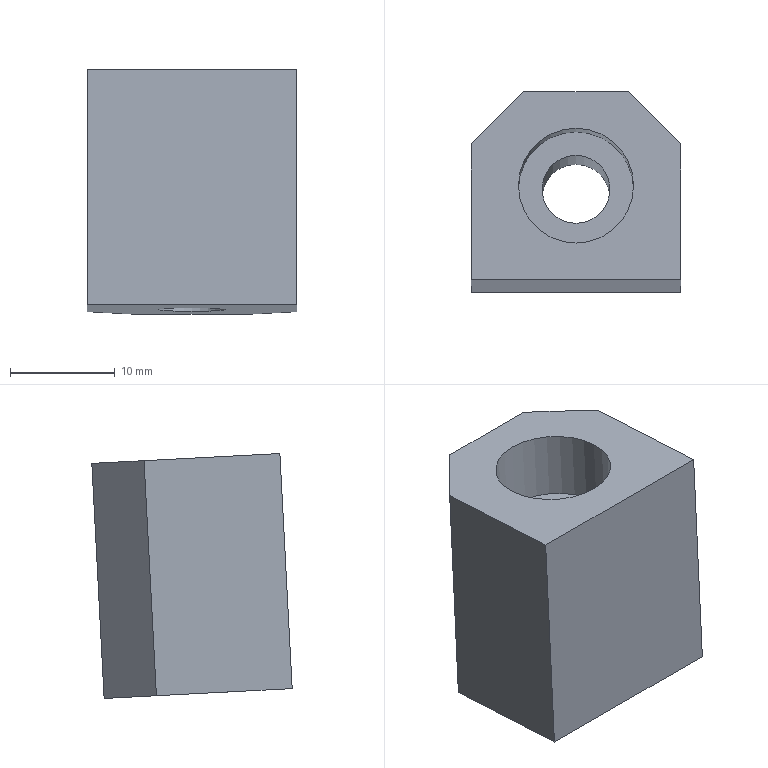Part | STEP file | P011002S001-007 | 1 solid | 11 faces | box 20 x 19.153 x 23.411 mm | volume 6389 mm3 | plane 9 | cylinder 2 | commonest cylinder face diameters 6.5 x1 11 x1
STEP:
#1=CARTESIAN_POINT('',(0.,0.,0.));
#2=DIRECTION('',(0.,0.,1.));
#3=DIRECTION('',(1.,0.,0.));
#4=AXIS2_PLACEMENT_3D('',#1,#2,#3);
#5=CARTESIAN_POINT('',(9.5,264.525,-24.398));
#6=VERTEX_POINT('',#5);
#7=CARTESIAN_POINT('',(9.5,277.507,-25.078));
#8=VERTEX_POINT('',#7);
#9=CARTESIAN_POINT('',(9.5,264.525,-24.398));
#10=DIRECTION('',(0.,0.9986,-0.05234));
#11=VECTOR('',#10,1.);
#12=LINE('',#9,#11);
#13=CARTESIAN_POINT('',(-5.5,264.525,-24.398));
#14=DIRECTION('',(0.,-0.05234,-0.9986));
#15=DIRECTION('',(0.,0.9986,-0.05234));
#16=AXIS2_PLACEMENT_3D('',#13,#14,#15);
#17=PLANE('',#16);
#18=CARTESIAN_POINT('',(0.,15.));
#19=DIRECTION('',(1.,0.));
#20=VECTOR('',#19,1.);
#21=LINE('',#18,#20);
#22=(GEOMETRIC_REPRESENTATION_CONTEXT(2)PARAMETRIC_REPRESENTATION_CONTEXT()REPRESENTATION_CONTEXT('',''));
#23=DEFINITIONAL_REPRESENTATION('',(#21),#22);
#24=PCURVE('',#17,#23);
#25=CARTESIAN_POINT('',(9.5,264.787,-19.405));
#26=DIRECTION('',(1.,0.,0.));
#27=DIRECTION('',(0.,-0.9986,0.05234));
#28=AXIS2_PLACEMENT_3D('',#25,#26,#27);
#29=PLANE('',#28);
#30=CARTESIAN_POINT('',(0.,5.));
#31=DIRECTION('',(-1.,0.));
#32=VECTOR('',#31,1.);
#33=LINE('',#30,#32);
#34=(GEOMETRIC_REPRESENTATION_CONTEXT(2)PARAMETRIC_REPRESENTATION_CONTEXT()REPRESENTATION_CONTEXT('',''));
#35=DEFINITIONAL_REPRESENTATION('',(#33),#34);
#36=PCURVE('',#29,#35);
#37=SURFACE_CURVE('',#12,(#24,#36),.PCURVE_S1.);
#38=EDGE_CURVE('',#6,#8,#37,.T.);
#39=ORIENTED_EDGE('',*,*,#38,.F.);
#40=CARTESIAN_POINT('',(-10.5,264.525,-24.398));
#41=VERTEX_POINT('',#40);
#42=CARTESIAN_POINT('',(-5.5,264.525,-24.398));
#43=DIRECTION('',(1.,0.,0.));
#44=VECTOR('',#43,1.);
#45=LINE('',#42,#44);
#46=CARTESIAN_POINT('',(0.,0.));
#47=DIRECTION('',(0.,1.));
#48=VECTOR('',#47,1.);
#49=LINE('',#46,#48);
#50=(GEOMETRIC_REPRESENTATION_CONTEXT(2)PARAMETRIC_REPRESENTATION_CONTEXT()REPRESENTATION_CONTEXT('',''));
#51=DEFINITIONAL_REPRESENTATION('',(#49),#50);
#52=PCURVE('',#17,#51);
#53=CARTESIAN_POINT('',(-5.5,264.787,-19.405));
#54=DIRECTION('',(0.,-0.9986,0.05234));
#55=DIRECTION('',(0.,-0.05234,-0.9986));
#56=AXIS2_PLACEMENT_3D('',#53,#54,#55);
#57=PLANE('',#56);
#58=CARTESIAN_POINT('',(5.,0.));
#59=DIRECTION('',(0.,1.));
#60=VECTOR('',#59,1.);
#61=LINE('',#58,#60);
#62=(GEOMETRIC_REPRESENTATION_CONTEXT(2)PARAMETRIC_REPRESENTATION_CONTEXT()REPRESENTATION_CONTEXT('',''));
#63=DEFINITIONAL_REPRESENTATION('',(#61),#62);
#64=PCURVE('',#57,#63);
#65=SURFACE_CURVE('',#45,(#52,#64),.PCURVE_S1.);
#66=EDGE_CURVE('',#41,#6,#65,.T.);
#67=ORIENTED_EDGE('',*,*,#66,.F.);
#68=CARTESIAN_POINT('',(-10.5,277.507,-25.078));
#69=VERTEX_POINT('',#68);
#70=CARTESIAN_POINT('',(-10.5,264.525,-24.398));
#71=DIRECTION('',(0.,0.9986,-0.05234));
#72=VECTOR('',#71,1.);
#73=LINE('',#70,#72);
#74=CARTESIAN_POINT('',(0.,-5.));
#75=DIRECTION('',(1.,0.));
#76=VECTOR('',#75,1.);
#77=LINE('',#74,#76);
#78=(GEOMETRIC_REPRESENTATION_CONTEXT(2)PARAMETRIC_REPRESENTATION_CONTEXT()REPRESENTATION_CONTEXT('',''));
#79=DEFINITIONAL_REPRESENTATION('',(#77),#78);
#80=PCURVE('',#17,#79);
#81=CARTESIAN_POINT('',(-10.5,264.787,-19.405));
#82=DIRECTION('',(-1.,0.,0.));
#83=DIRECTION('',(0.,0.9986,-0.05234));
#84=AXIS2_PLACEMENT_3D('',#81,#82,#83);
#85=PLANE('',#84);
#86=CARTESIAN_POINT('',(0.,5.));
#87=DIRECTION('',(1.,0.));
#88=VECTOR('',#87,1.);
#89=LINE('',#86,#88);
#90=(GEOMETRIC_REPRESENTATION_CONTEXT(2)PARAMETRIC_REPRESENTATION_CONTEXT()REPRESENTATION_CONTEXT('',''));
#91=DEFINITIONAL_REPRESENTATION('',(#89),#90);
#92=PCURVE('',#85,#91);
#93=SURFACE_CURVE('',#73,(#80,#92),.PCURVE_S1.);
#94=EDGE_CURVE('',#41,#69,#93,.T.);
#95=ORIENTED_EDGE('',*,*,#94,.T.);
#96=CARTESIAN_POINT('',(-5.5,282.5,-25.34));
#97=VERTEX_POINT('',#96);
#98=CARTESIAN_POINT('',(-14.5,273.513,-24.869));
#99=DIRECTION('',(-0.7071,-0.7061,0.03701));
#100=VECTOR('',#99,1.);
#101=LINE('',#98,#100);
#102=CARTESIAN_POINT('',(9.,-9.));
#103=DIRECTION('',(-0.7071,-0.7071));
#104=VECTOR('',#103,1.);
#105=LINE('',#102,#104);
#106=(GEOMETRIC_REPRESENTATION_CONTEXT(2)PARAMETRIC_REPRESENTATION_CONTEXT()REPRESENTATION_CONTEXT('',''));
#107=DEFINITIONAL_REPRESENTATION('',(#105),#106);
#108=PCURVE('',#17,#107);
#109=CARTESIAN_POINT('',(-10.5,277.769,-20.085));
#110=DIRECTION('',(0.7071,-0.7061,0.03701));
#111=DIRECTION('',(-0.7066,-0.7076,0.));
#112=AXIS2_PLACEMENT_3D('',#109,#110,#111);
#113=PLANE('',#112);
#114=CARTESIAN_POINT('',(5.838,4.787));
#115=DIRECTION('',(0.9993,-0.03703));
#116=VECTOR('',#115,1.);
#117=LINE('',#114,#116);
#118=(GEOMETRIC_REPRESENTATION_CONTEXT(2)PARAMETRIC_REPRESENTATION_CONTEXT()REPRESENTATION_CONTEXT('',''));
#119=DEFINITIONAL_REPRESENTATION('',(#117),#118);
#120=PCURVE('',#113,#119);
#121=SURFACE_CURVE('',#101,(#108,#120),.PCURVE_S1.);
#122=EDGE_CURVE('',#97,#69,#121,.T.);
#123=ORIENTED_EDGE('',*,*,#122,.F.);
#124=CARTESIAN_POINT('',(4.5,282.5,-25.34));
#125=VERTEX_POINT('',#124);
#126=CARTESIAN_POINT('',(-5.5,282.5,-25.34));
#127=DIRECTION('',(-1.,0.,0.));
#128=VECTOR('',#127,1.);
#129=LINE('',#126,#128);
#130=CARTESIAN_POINT('',(18.,0.));
#131=DIRECTION('',(0.,-1.));
#132=VECTOR('',#131,1.);
#133=LINE('',#130,#132);
#134=(GEOMETRIC_REPRESENTATION_CONTEXT(2)PARAMETRIC_REPRESENTATION_CONTEXT()REPRESENTATION_CONTEXT('',''));
#135=DEFINITIONAL_REPRESENTATION('',(#133),#134);
#136=PCURVE('',#17,#135);
#137=CARTESIAN_POINT('',(-5.5,282.762,-20.347));
#138=DIRECTION('',(0.,0.9986,-0.05234));
#139=DIRECTION('',(0.,0.05234,0.9986));
#140=AXIS2_PLACEMENT_3D('',#137,#138,#139);
#141=PLANE('',#140);
#142=CARTESIAN_POINT('',(-5.,0.));
#143=DIRECTION('',(0.,-1.));
#144=VECTOR('',#143,1.);
#145=LINE('',#142,#144);
#146=(GEOMETRIC_REPRESENTATION_CONTEXT(2)PARAMETRIC_REPRESENTATION_CONTEXT()REPRESENTATION_CONTEXT('',''));
#147=DEFINITIONAL_REPRESENTATION('',(#145),#146);
#148=PCURVE('',#141,#147);
#149=SURFACE_CURVE('',#129,(#136,#148),.PCURVE_S1.);
#150=EDGE_CURVE('',#125,#97,#149,.T.);
#151=ORIENTED_EDGE('',*,*,#150,.F.);
#152=CARTESIAN_POINT('',(8.5,278.506,-25.131));
#153=DIRECTION('',(-0.7071,0.7061,-0.03701));
#154=VECTOR('',#153,1.);
#155=LINE('',#152,#154);
#156=CARTESIAN_POINT('',(14.,14.));
#157=DIRECTION('',(0.7071,-0.7071));
#158=VECTOR('',#157,1.);
#159=LINE('',#156,#158);
#160=(GEOMETRIC_REPRESENTATION_CONTEXT(2)PARAMETRIC_REPRESENTATION_CONTEXT()REPRESENTATION_CONTEXT('',''));
#161=DEFINITIONAL_REPRESENTATION('',(#159),#160);
#162=PCURVE('',#17,#161);
#163=CARTESIAN_POINT('',(9.5,277.769,-20.085));
#164=DIRECTION('',(-0.7071,-0.7061,0.03701));
#165=DIRECTION('',(-0.7066,0.7076,0.));
#166=AXIS2_PLACEMENT_3D('',#163,#164,#165);
#167=PLANE('',#166);
#168=CARTESIAN_POINT('',(1.228,5.049));
#169=DIRECTION('',(0.9993,0.03703));
#170=VECTOR('',#169,1.);
#171=LINE('',#168,#170);
#172=(GEOMETRIC_REPRESENTATION_CONTEXT(2)PARAMETRIC_REPRESENTATION_CONTEXT()REPRESENTATION_CONTEXT('',''));
#173=DEFINITIONAL_REPRESENTATION('',(#171),#172);
#174=PCURVE('',#167,#173);
#175=SURFACE_CURVE('',#155,(#162,#174),.PCURVE_S1.);
#176=EDGE_CURVE('',#8,#125,#175,.T.);
#177=ORIENTED_EDGE('',*,*,#176,.F.);
#178=EDGE_LOOP('',(#39,#67,#95,#123,#151,#177));
#179=FACE_BOUND('',#178,.T.);
#180=CARTESIAN_POINT('',(-0.5,276.758,-25.039));
#181=VERTEX_POINT('',#180);
#182=CARTESIAN_POINT('',(-0.5,273.513,-24.869));
#183=DIRECTION('',(0.,-0.05234,-0.9986));
#184=DIRECTION('',(0.,0.9986,-0.05234));
#185=AXIS2_PLACEMENT_3D('',#182,#183,#184);
#186=CIRCLE('',#185,3.25);
#187=CARTESIAN_POINT('',(9.,5.));
#188=DIRECTION('',(1.,0.));
#189=AXIS2_PLACEMENT_2D('',#187,#188);
#190=CIRCLE('',#189,3.25);
#191=(GEOMETRIC_REPRESENTATION_CONTEXT(2)PARAMETRIC_REPRESENTATION_CONTEXT()REPRESENTATION_CONTEXT('',''));
#192=DEFINITIONAL_REPRESENTATION('',(#190),#191);
#193=PCURVE('',#17,#192);
#194=CARTESIAN_POINT('',(-0.5,274.69,-2.4));
#195=DIRECTION('',(0.,-0.05234,-0.9986));
#196=DIRECTION('',(0.,0.9986,-0.05234));
#197=AXIS2_PLACEMENT_3D('',#194,#195,#196);
#198=CYLINDRICAL_SURFACE('',#197,3.25);
#199=CARTESIAN_POINT('',(0.,22.5));
#200=DIRECTION('',(1.,0.));
#201=VECTOR('',#200,1.);
#202=LINE('',#199,#201);
#203=(GEOMETRIC_REPRESENTATION_CONTEXT(2)PARAMETRIC_REPRESENTATION_CONTEXT()REPRESENTATION_CONTEXT('',''));
#204=DEFINITIONAL_REPRESENTATION('',(#202),#203);
#205=PCURVE('',#198,#204);
#206=SURFACE_CURVE('',#186,(#193,#205),.PCURVE_S1.);
#207=EDGE_CURVE('',#181,#181,#206,.T.);
#208=ORIENTED_EDGE('',*,*,#207,.F.);
#209=EDGE_LOOP('',(#208));
#210=FACE_BOUND('',#209,.T.);
#211=ADVANCED_FACE('',(#179,#210),#17,.T.);
#212=ORIENTED_EDGE('',*,*,#150,.T.);
#213=CARTESIAN_POINT('',(-5.5,283.678,-2.871));
#214=VERTEX_POINT('',#213);
#215=CARTESIAN_POINT('',(-5.5,282.762,-20.347));
#216=DIRECTION('',(0.,-0.05234,-0.9986));
#217=VECTOR('',#216,1.);
#218=LINE('',#215,#217);
#219=CARTESIAN_POINT('',(0.,0.));
#220=DIRECTION('',(-1.,0.));
#221=VECTOR('',#220,1.);
#222=LINE('',#219,#221);
#223=(GEOMETRIC_REPRESENTATION_CONTEXT(2)PARAMETRIC_REPRESENTATION_CONTEXT()REPRESENTATION_CONTEXT('',''));
#224=DEFINITIONAL_REPRESENTATION('',(#222),#223);
#225=PCURVE('',#141,#224);
#226=CARTESIAN_POINT('',(-7.066,0.2619));
#227=DIRECTION('',(0.03703,0.9993));
#228=VECTOR('',#227,1.);
#229=LINE('',#226,#228);
#230=(GEOMETRIC_REPRESENTATION_CONTEXT(2)PARAMETRIC_REPRESENTATION_CONTEXT()REPRESENTATION_CONTEXT('',''));
#231=DEFINITIONAL_REPRESENTATION('',(#229),#230);
#232=PCURVE('',#113,#231);
#233=SURFACE_CURVE('',#218,(#225,#232),.PCURVE_S1.);
#234=EDGE_CURVE('',#214,#97,#233,.T.);
#235=ORIENTED_EDGE('',*,*,#234,.F.);
#236=CARTESIAN_POINT('',(4.5,283.678,-2.871));
#237=VERTEX_POINT('',#236);
#238=CARTESIAN_POINT('',(-5.5,283.678,-2.871));
#239=DIRECTION('',(1.,0.,0.));
#240=VECTOR('',#239,1.);
#241=LINE('',#238,#240);
#242=CARTESIAN_POINT('',(17.5,0.));
#243=DIRECTION('',(0.,1.));
#244=VECTOR('',#243,1.);
#245=LINE('',#242,#244);
#246=(GEOMETRIC_REPRESENTATION_CONTEXT(2)PARAMETRIC_REPRESENTATION_CONTEXT()REPRESENTATION_CONTEXT('',''));
#247=DEFINITIONAL_REPRESENTATION('',(#245),#246);
#248=PCURVE('',#141,#247);
#249=CARTESIAN_POINT('',(-5.5,265.703,-1.929));
#250=DIRECTION('',(0.,0.05234,0.9986));
#251=DIRECTION('',(0.,-0.9986,0.05234));
#252=AXIS2_PLACEMENT_3D('',#249,#250,#251);
#253=PLANE('',#252);
#254=CARTESIAN_POINT('',(-18.,0.));
#255=DIRECTION('',(0.,1.));
#256=VECTOR('',#255,1.);
#257=LINE('',#254,#256);
#258=(GEOMETRIC_REPRESENTATION_CONTEXT(2)PARAMETRIC_REPRESENTATION_CONTEXT()REPRESENTATION_CONTEXT('',''));
#259=DEFINITIONAL_REPRESENTATION('',(#257),#258);
#260=PCURVE('',#253,#259);
#261=SURFACE_CURVE('',#241,(#248,#260),.PCURVE_S1.);
#262=EDGE_CURVE('',#214,#237,#261,.T.);
#263=ORIENTED_EDGE('',*,*,#262,.T.);
#264=CARTESIAN_POINT('',(4.5,282.762,-20.347));
#265=DIRECTION('',(0.,0.05234,0.9986));
#266=VECTOR('',#265,1.);
#267=LINE('',#264,#266);
#268=CARTESIAN_POINT('',(0.,10.));
#269=DIRECTION('',(1.,0.));
#270=VECTOR('',#269,1.);
#271=LINE('',#268,#270);
#272=(GEOMETRIC_REPRESENTATION_CONTEXT(2)PARAMETRIC_REPRESENTATION_CONTEXT()REPRESENTATION_CONTEXT('',''));
#273=DEFINITIONAL_REPRESENTATION('',(#271),#272);
#274=PCURVE('',#141,#273);
#275=CARTESIAN_POINT('',(7.066,0.2619));
#276=DIRECTION('',(0.03703,-0.9993));
#277=VECTOR('',#276,1.);
#278=LINE('',#275,#277);
#279=(GEOMETRIC_REPRESENTATION_CONTEXT(2)PARAMETRIC_REPRESENTATION_CONTEXT()REPRESENTATION_CONTEXT('',''));
#280=DEFINITIONAL_REPRESENTATION('',(#278),#279);
#281=PCURVE('',#167,#280);
#282=SURFACE_CURVE('',#267,(#274,#281),.PCURVE_S1.);
#283=EDGE_CURVE('',#125,#237,#282,.T.);
#284=ORIENTED_EDGE('',*,*,#283,.F.);
#285=EDGE_LOOP('',(#212,#235,#263,#284));
#286=FACE_BOUND('',#285,.T.);
#287=ADVANCED_FACE('',(#286),#141,.T.);
#288=CARTESIAN_POINT('',(9.5,265.703,-1.929));
#289=VERTEX_POINT('',#288);
#290=CARTESIAN_POINT('',(9.5,278.685,-2.609));
#291=VERTEX_POINT('',#290);
#292=CARTESIAN_POINT('',(9.5,265.703,-1.929));
#293=DIRECTION('',(0.,0.9986,-0.05234));
#294=VECTOR('',#293,1.);
#295=LINE('',#292,#294);
#296=CARTESIAN_POINT('',(0.,-17.5));
#297=DIRECTION('',(-1.,0.));
#298=VECTOR('',#297,1.);
#299=LINE('',#296,#298);
#300=(GEOMETRIC_REPRESENTATION_CONTEXT(2)PARAMETRIC_REPRESENTATION_CONTEXT()REPRESENTATION_CONTEXT('',''));
#301=DEFINITIONAL_REPRESENTATION('',(#299),#300);
#302=PCURVE('',#29,#301);
#303=CARTESIAN_POINT('',(0.,15.));
#304=DIRECTION('',(-1.,0.));
#305=VECTOR('',#304,1.);
#306=LINE('',#303,#305);
#307=(GEOMETRIC_REPRESENTATION_CONTEXT(2)PARAMETRIC_REPRESENTATION_CONTEXT()REPRESENTATION_CONTEXT('',''));
#308=DEFINITIONAL_REPRESENTATION('',(#306),#307);
#309=PCURVE('',#253,#308);
#310=SURFACE_CURVE('',#295,(#302,#309),.PCURVE_S1.);
#311=EDGE_CURVE('',#289,#291,#310,.T.);
#312=ORIENTED_EDGE('',*,*,#311,.F.);
#313=CARTESIAN_POINT('',(9.5,264.787,-19.405));
#314=DIRECTION('',(0.,0.05234,0.9986));
#315=VECTOR('',#314,1.);
#316=LINE('',#313,#315);
#317=CARTESIAN_POINT('',(0.,0.));
#318=DIRECTION('',(0.,-1.));
#319=VECTOR('',#318,1.);
#320=LINE('',#317,#319);
#321=(GEOMETRIC_REPRESENTATION_CONTEXT(2)PARAMETRIC_REPRESENTATION_CONTEXT()REPRESENTATION_CONTEXT('',''));
#322=DEFINITIONAL_REPRESENTATION('',(#320),#321);
#323=PCURVE('',#29,#322);
#324=CARTESIAN_POINT('',(0.,15.));
#325=DIRECTION('',(-1.,0.));
#326=VECTOR('',#325,1.);
#327=LINE('',#324,#326);
#328=(GEOMETRIC_REPRESENTATION_CONTEXT(2)PARAMETRIC_REPRESENTATION_CONTEXT()REPRESENTATION_CONTEXT('',''));
#329=DEFINITIONAL_REPRESENTATION('',(#327),#328);
#330=PCURVE('',#57,#329);
#331=SURFACE_CURVE('',#316,(#323,#330),.PCURVE_S1.);
#332=EDGE_CURVE('',#6,#289,#331,.T.);
#333=ORIENTED_EDGE('',*,*,#332,.F.);
#334=ORIENTED_EDGE('',*,*,#38,.T.);
#335=CARTESIAN_POINT('',(9.5,277.769,-20.085));
#336=DIRECTION('',(0.,-0.05234,-0.9986));
#337=VECTOR('',#336,1.);
#338=LINE('',#335,#337);
#339=CARTESIAN_POINT('',(-13.,0.));
#340=DIRECTION('',(0.,1.));
#341=VECTOR('',#340,1.);
#342=LINE('',#339,#341);
#343=(GEOMETRIC_REPRESENTATION_CONTEXT(2)PARAMETRIC_REPRESENTATION_CONTEXT()REPRESENTATION_CONTEXT('',''));
#344=DEFINITIONAL_REPRESENTATION('',(#342),#343);
#345=PCURVE('',#29,#344);
#346=CARTESIAN_POINT('',(0.,0.));
#347=DIRECTION('',(-0.03703,0.9993));
#348=VECTOR('',#347,1.);
#349=LINE('',#346,#348);
#350=(GEOMETRIC_REPRESENTATION_CONTEXT(2)PARAMETRIC_REPRESENTATION_CONTEXT()REPRESENTATION_CONTEXT('',''));
#351=DEFINITIONAL_REPRESENTATION('',(#349),#350);
#352=PCURVE('',#167,#351);
#353=SURFACE_CURVE('',#338,(#345,#352),.PCURVE_S1.);
#354=EDGE_CURVE('',#291,#8,#353,.T.);
#355=ORIENTED_EDGE('',*,*,#354,.F.);
#356=EDGE_LOOP('',(#312,#333,#334,#355));
#357=FACE_BOUND('',#356,.T.);
#358=ADVANCED_FACE('',(#357),#29,.T.);
#359=ORIENTED_EDGE('',*,*,#94,.F.);
#360=CARTESIAN_POINT('',(-10.5,265.703,-1.929));
#361=VERTEX_POINT('',#360);
#362=CARTESIAN_POINT('',(-10.5,264.787,-19.405));
#363=DIRECTION('',(0.,-0.05234,-0.9986));
#364=VECTOR('',#363,1.);
#365=LINE('',#362,#364);
#366=CARTESIAN_POINT('',(0.,0.));
#367=DIRECTION('',(0.,1.));
#368=VECTOR('',#367,1.);
#369=LINE('',#366,#368);
#370=(GEOMETRIC_REPRESENTATION_CONTEXT(2)PARAMETRIC_REPRESENTATION_CONTEXT()REPRESENTATION_CONTEXT('',''));
#371=DEFINITIONAL_REPRESENTATION('',(#369),#370);
#372=PCURVE('',#85,#371);
#373=CARTESIAN_POINT('',(0.,-5.));
#374=DIRECTION('',(1.,0.));
#375=VECTOR('',#374,1.);
#376=LINE('',#373,#375);
#377=(GEOMETRIC_REPRESENTATION_CONTEXT(2)PARAMETRIC_REPRESENTATION_CONTEXT()REPRESENTATION_CONTEXT('',''));
#378=DEFINITIONAL_REPRESENTATION('',(#376),#377);
#379=PCURVE('',#57,#378);
#380=SURFACE_CURVE('',#365,(#372,#379),.PCURVE_S1.);
#381=EDGE_CURVE('',#361,#41,#380,.T.);
#382=ORIENTED_EDGE('',*,*,#381,.F.);
#383=CARTESIAN_POINT('',(-10.5,278.685,-2.609));
#384=VERTEX_POINT('',#383);
#385=CARTESIAN_POINT('',(-10.5,265.703,-1.929));
#386=DIRECTION('',(0.,0.9986,-0.05234));
#387=VECTOR('',#386,1.);
#388=LINE('',#385,#387);
#389=CARTESIAN_POINT('',(0.,-17.5));
#390=DIRECTION('',(1.,0.));
#391=VECTOR('',#390,1.);
#392=LINE('',#389,#391);
#393=(GEOMETRIC_REPRESENTATION_CONTEXT(2)PARAMETRIC_REPRESENTATION_CONTEXT()REPRESENTATION_CONTEXT('',''));
#394=DEFINITIONAL_REPRESENTATION('',(#392),#393);
#395=PCURVE('',#85,#394);
#396=CARTESIAN_POINT('',(0.,-5.));
#397=DIRECTION('',(-1.,0.));
#398=VECTOR('',#397,1.);
#399=LINE('',#396,#398);
#400=(GEOMETRIC_REPRESENTATION_CONTEXT(2)PARAMETRIC_REPRESENTATION_CONTEXT()REPRESENTATION_CONTEXT('',''));
#401=DEFINITIONAL_REPRESENTATION('',(#399),#400);
#402=PCURVE('',#253,#401);
#403=SURFACE_CURVE('',#388,(#395,#402),.PCURVE_S1.);
#404=EDGE_CURVE('',#361,#384,#403,.T.);
#405=ORIENTED_EDGE('',*,*,#404,.T.);
#406=CARTESIAN_POINT('',(-10.5,277.769,-20.085));
#407=DIRECTION('',(0.,0.05234,0.9986));
#408=VECTOR('',#407,1.);
#409=LINE('',#406,#408);
#410=CARTESIAN_POINT('',(13.,0.));
#411=DIRECTION('',(0.,-1.));
#412=VECTOR('',#411,1.);
#413=LINE('',#410,#412);
#414=(GEOMETRIC_REPRESENTATION_CONTEXT(2)PARAMETRIC_REPRESENTATION_CONTEXT()REPRESENTATION_CONTEXT('',''));
#415=DEFINITIONAL_REPRESENTATION('',(#413),#414);
#416=PCURVE('',#85,#415);
#417=CARTESIAN_POINT('',(0.,0.));
#418=DIRECTION('',(-0.03703,-0.9993));
#419=VECTOR('',#418,1.);
#420=LINE('',#417,#419);
#421=(GEOMETRIC_REPRESENTATION_CONTEXT(2)PARAMETRIC_REPRESENTATION_CONTEXT()REPRESENTATION_CONTEXT('',''));
#422=DEFINITIONAL_REPRESENTATION('',(#420),#421);
#423=PCURVE('',#113,#422);
#424=SURFACE_CURVE('',#409,(#416,#423),.PCURVE_S1.);
#425=EDGE_CURVE('',#69,#384,#424,.T.);
#426=ORIENTED_EDGE('',*,*,#425,.F.);
#427=EDGE_LOOP('',(#359,#382,#405,#426));
#428=FACE_BOUND('',#427,.T.);
#429=ADVANCED_FACE('',(#428),#85,.T.);
#430=CARTESIAN_POINT('',(-5.5,265.703,-1.929));
#431=DIRECTION('',(-1.,0.,0.));
#432=VECTOR('',#431,1.);
#433=LINE('',#430,#432);
#434=CARTESIAN_POINT('',(-17.5,0.));
#435=DIRECTION('',(0.,-1.));
#436=VECTOR('',#435,1.);
#437=LINE('',#434,#436);
#438=(GEOMETRIC_REPRESENTATION_CONTEXT(2)PARAMETRIC_REPRESENTATION_CONTEXT()REPRESENTATION_CONTEXT('',''));
#439=DEFINITIONAL_REPRESENTATION('',(#437),#438);
#440=PCURVE('',#57,#439);
#441=CARTESIAN_POINT('',(0.,0.));
#442=DIRECTION('',(0.,-1.));
#443=VECTOR('',#442,1.);
#444=LINE('',#441,#443);
#445=(GEOMETRIC_REPRESENTATION_CONTEXT(2)PARAMETRIC_REPRESENTATION_CONTEXT()REPRESENTATION_CONTEXT('',''));
#446=DEFINITIONAL_REPRESENTATION('',(#444),#445);
#447=PCURVE('',#253,#446);
#448=SURFACE_CURVE('',#433,(#440,#447),.PCURVE_S1.);
#449=EDGE_CURVE('',#289,#361,#448,.T.);
#450=ORIENTED_EDGE('',*,*,#449,.T.);
#451=ORIENTED_EDGE('',*,*,#381,.T.);
#452=ORIENTED_EDGE('',*,*,#66,.T.);
#453=ORIENTED_EDGE('',*,*,#332,.T.);
#454=EDGE_LOOP('',(#450,#451,#452,#453));
#455=FACE_BOUND('',#454,.T.);
#456=ADVANCED_FACE('',(#455),#57,.T.);
#457=CARTESIAN_POINT('',(-0.5,269.198,-2.112));
#458=VERTEX_POINT('',#457);
#459=CARTESIAN_POINT('',(-0.5,280.183,-2.688));
#460=VERTEX_POINT('',#459);
#461=CARTESIAN_POINT('',(-0.5,274.69,-2.4));
#462=DIRECTION('',(0.,-0.05234,-0.9986));
#463=DIRECTION('',(0.,-0.9986,0.05234));
#464=AXIS2_PLACEMENT_3D('',#461,#462,#463);
#465=CIRCLE('',#464,5.5);
#466=CARTESIAN_POINT('',(-3.5,5.));
#467=CARTESIAN_POINT('',(-3.5,-4.526));
#468=CARTESIAN_POINT('',(-11.75,0.2369));
#469=CARTESIAN_POINT('',(-20.,5.));
#470=CARTESIAN_POINT('',(-11.75,9.763));
#471=CARTESIAN_POINT('',(-3.5,14.526));
#472=CARTESIAN_POINT('',(-3.5,5.));
#473=(BOUNDED_CURVE()B_SPLINE_CURVE(2,(#466,#467,#468,#469,#470,#471,#472),.UNSPECIFIED.,.T.,.F.)B_SPLINE_CURVE_WITH_KNOTS((1,2,2,2,2,1),(-2.094,0.,2.094,4.189,6.283,8.378),.UNSPECIFIED.)CURVE()GEOMETRIC_REPRESENTATION_ITEM()RATIONAL_B_SPLINE_CURVE((1.,0.5,1.,0.5,1.,0.5,1.))REPRESENTATION_ITEM(''));
#474=(GEOMETRIC_REPRESENTATION_CONTEXT(2)PARAMETRIC_REPRESENTATION_CONTEXT()REPRESENTATION_CONTEXT('',''));
#475=DEFINITIONAL_REPRESENTATION('',(#473),#474);
#476=PCURVE('',#253,#475);
#477=CARTESIAN_POINT('',(-0.5,274.69,-2.4));
#478=DIRECTION('',(0.,-0.05234,-0.9986));
#479=DIRECTION('',(0.,0.9986,-0.05234));
#480=AXIS2_PLACEMENT_3D('',#477,#478,#479);
#481=CYLINDRICAL_SURFACE('',#480,5.5);
#482=CARTESIAN_POINT('',(3.142,0.));
#483=DIRECTION('',(1.,0.));
#484=VECTOR('',#483,1.);
#485=LINE('',#482,#484);
#486=(GEOMETRIC_REPRESENTATION_CONTEXT(2)PARAMETRIC_REPRESENTATION_CONTEXT()REPRESENTATION_CONTEXT('',''));
#487=DEFINITIONAL_REPRESENTATION('',(#485),#486);
#488=PCURVE('',#481,#487);
#489=SURFACE_CURVE('',#465,(#476,#488),.PCURVE_S1.);
#490=EDGE_CURVE('',#458,#460,#489,.T.);
#491=ORIENTED_EDGE('',*,*,#490,.T.);
#492=CARTESIAN_POINT('',(-0.5,274.69,-2.4));
#493=DIRECTION('',(0.,-0.05234,-0.9986));
#494=DIRECTION('',(0.,-0.9986,0.05234));
#495=AXIS2_PLACEMENT_3D('',#492,#493,#494);
#496=CIRCLE('',#495,5.5);
#497=CARTESIAN_POINT('',(-3.5,5.));
#498=CARTESIAN_POINT('',(-3.5,-4.526));
#499=CARTESIAN_POINT('',(-11.75,0.2369));
#500=CARTESIAN_POINT('',(-20.,5.));
#501=CARTESIAN_POINT('',(-11.75,9.763));
#502=CARTESIAN_POINT('',(-3.5,14.526));
#503=CARTESIAN_POINT('',(-3.5,5.));
#504=(BOUNDED_CURVE()B_SPLINE_CURVE(2,(#497,#498,#499,#500,#501,#502,#503),.UNSPECIFIED.,.T.,.F.)B_SPLINE_CURVE_WITH_KNOTS((1,2,2,2,2,1),(-2.094,0.,2.094,4.189,6.283,8.378),.UNSPECIFIED.)CURVE()GEOMETRIC_REPRESENTATION_ITEM()RATIONAL_B_SPLINE_CURVE((1.,0.5,1.,0.5,1.,0.5,1.))REPRESENTATION_ITEM(''));
#505=(GEOMETRIC_REPRESENTATION_CONTEXT(2)PARAMETRIC_REPRESENTATION_CONTEXT()REPRESENTATION_CONTEXT('',''));
#506=DEFINITIONAL_REPRESENTATION('',(#504),#505);
#507=PCURVE('',#253,#506);
#508=CARTESIAN_POINT('',(-3.142,0.));
#509=DIRECTION('',(1.,0.));
#510=VECTOR('',#509,1.);
#511=LINE('',#508,#510);
#512=(GEOMETRIC_REPRESENTATION_CONTEXT(2)PARAMETRIC_REPRESENTATION_CONTEXT()REPRESENTATION_CONTEXT('',''));
#513=DEFINITIONAL_REPRESENTATION('',(#511),#512);
#514=PCURVE('',#481,#513);
#515=SURFACE_CURVE('',#496,(#507,#514),.PCURVE_S1.);
#516=EDGE_CURVE('',#460,#458,#515,.T.);
#517=ORIENTED_EDGE('',*,*,#516,.T.);
#518=EDGE_LOOP('',(#491,#517));
#519=FACE_BOUND('',#518,.T.);
#520=ORIENTED_EDGE('',*,*,#262,.F.);
#521=CARTESIAN_POINT('',(-14.5,274.69,-2.4));
#522=DIRECTION('',(0.7071,0.7061,-0.03701));
#523=VECTOR('',#522,1.);
#524=LINE('',#521,#523);
#525=CARTESIAN_POINT('',(-9.,-9.));
#526=DIRECTION('',(-0.7071,0.7071));
#527=VECTOR('',#526,1.);
#528=LINE('',#525,#527);
#529=(GEOMETRIC_REPRESENTATION_CONTEXT(2)PARAMETRIC_REPRESENTATION_CONTEXT()REPRESENTATION_CONTEXT('',''));
#530=DEFINITIONAL_REPRESENTATION('',(#528),#529);
#531=PCURVE('',#253,#530);
#532=CARTESIAN_POINT('',(5.005,-17.697));
#533=DIRECTION('',(-0.9993,0.03703));
#534=VECTOR('',#533,1.);
#535=LINE('',#532,#534);
#536=(GEOMETRIC_REPRESENTATION_CONTEXT(2)PARAMETRIC_REPRESENTATION_CONTEXT()REPRESENTATION_CONTEXT('',''));
#537=DEFINITIONAL_REPRESENTATION('',(#535),#536);
#538=PCURVE('',#113,#537);
#539=SURFACE_CURVE('',#524,(#531,#538),.PCURVE_S1.);
#540=EDGE_CURVE('',#384,#214,#539,.T.);
#541=ORIENTED_EDGE('',*,*,#540,.F.);
#542=ORIENTED_EDGE('',*,*,#404,.F.);
#543=ORIENTED_EDGE('',*,*,#449,.F.);
#544=ORIENTED_EDGE('',*,*,#311,.T.);
#545=CARTESIAN_POINT('',(8.5,279.683,-2.662));
#546=DIRECTION('',(0.7071,-0.7061,0.03701));
#547=VECTOR('',#546,1.);
#548=LINE('',#545,#547);
#549=CARTESIAN_POINT('',(-14.,14.));
#550=DIRECTION('',(0.7071,0.7071));
#551=VECTOR('',#550,1.);
#552=LINE('',#549,#551);
#553=(GEOMETRIC_REPRESENTATION_CONTEXT(2)PARAMETRIC_REPRESENTATION_CONTEXT()REPRESENTATION_CONTEXT('',''));
#554=DEFINITIONAL_REPRESENTATION('',(#552),#553);
#555=PCURVE('',#253,#554);
#556=CARTESIAN_POINT('',(2.061,-17.436));
#557=DIRECTION('',(-0.9993,-0.03703));
#558=VECTOR('',#557,1.);
#559=LINE('',#556,#558);
#560=(GEOMETRIC_REPRESENTATION_CONTEXT(2)PARAMETRIC_REPRESENTATION_CONTEXT()REPRESENTATION_CONTEXT('',''));
#561=DEFINITIONAL_REPRESENTATION('',(#559),#560);
#562=PCURVE('',#167,#561);
#563=SURFACE_CURVE('',#548,(#555,#562),.PCURVE_S1.);
#564=EDGE_CURVE('',#237,#291,#563,.T.);
#565=ORIENTED_EDGE('',*,*,#564,.F.);
#566=EDGE_LOOP('',(#520,#541,#542,#543,#544,#565));
#567=FACE_BOUND('',#566,.T.);
#568=ADVANCED_FACE('',(#519,#567),#253,.T.);
#569=ORIENTED_EDGE('',*,*,#564,.T.);
#570=ORIENTED_EDGE('',*,*,#354,.T.);
#571=ORIENTED_EDGE('',*,*,#176,.T.);
#572=ORIENTED_EDGE('',*,*,#283,.T.);
#573=EDGE_LOOP('',(#569,#570,#571,#572));
#574=FACE_BOUND('',#573,.T.);
#575=ADVANCED_FACE('',(#574),#167,.F.);
#576=ORIENTED_EDGE('',*,*,#122,.T.);
#577=ORIENTED_EDGE('',*,*,#425,.T.);
#578=ORIENTED_EDGE('',*,*,#540,.T.);
#579=ORIENTED_EDGE('',*,*,#234,.T.);
#580=EDGE_LOOP('',(#576,#577,#578,#579));
#581=FACE_BOUND('',#580,.T.);
#582=ADVANCED_FACE('',(#581),#113,.F.);
#583=ORIENTED_EDGE('',*,*,#207,.F.);
#584=CARTESIAN_POINT('',(-0.5,277.596,-9.061));
#585=VERTEX_POINT('',#584);
#586=CARTESIAN_POINT('',(-0.5,277.596,-9.061));
#587=CARTESIAN_POINT('',(-0.5,276.758,-25.039));
#588=B_SPLINE_CURVE_WITH_KNOTS('',1,(#586,#587),.UNSPECIFIED.,.F.,.F.,(2,2),(6.5,22.5),.PIECEWISE_BEZIER_KNOTS.);
#589=CARTESIAN_POINT('',(0.,0.));
#590=DIRECTION('',(0.,1.));
#591=VECTOR('',#590,1.);
#592=LINE('',#589,#591);
#593=(GEOMETRIC_REPRESENTATION_CONTEXT(2)PARAMETRIC_REPRESENTATION_CONTEXT()REPRESENTATION_CONTEXT('',''));
#594=DEFINITIONAL_REPRESENTATION('',(#592),#593);
#595=PCURVE('',#198,#594);
#596=CARTESIAN_POINT('',(6.283,0.));
#597=DIRECTION('',(0.,1.));
#598=VECTOR('',#597,1.);
#599=LINE('',#596,#598);
#600=(GEOMETRIC_REPRESENTATION_CONTEXT(2)PARAMETRIC_REPRESENTATION_CONTEXT()REPRESENTATION_CONTEXT('',''));
#601=DEFINITIONAL_REPRESENTATION('',(#599),#600);
#602=PCURVE('',#198,#601);
#603=SEAM_CURVE('',#588,(#595,#602),.PCURVE_S1.);
#604=EDGE_CURVE('',#585,#181,#603,.T.);
#605=ORIENTED_EDGE('',*,*,#604,.F.);
#606=CARTESIAN_POINT('',(-0.5,274.35,-8.891));
#607=DIRECTION('',(0.,0.05234,0.9986));
#608=DIRECTION('',(0.,0.9986,-0.05234));
#609=AXIS2_PLACEMENT_3D('',#606,#607,#608);
#610=CIRCLE('',#609,3.25);
#611=CARTESIAN_POINT('',(6.283,6.5));
#612=DIRECTION('',(-1.,0.));
#613=VECTOR('',#612,1.);
#614=LINE('',#611,#613);
#615=(GEOMETRIC_REPRESENTATION_CONTEXT(2)PARAMETRIC_REPRESENTATION_CONTEXT()REPRESENTATION_CONTEXT('',''));
#616=DEFINITIONAL_REPRESENTATION('',(#614),#615);
#617=PCURVE('',#198,#616);
#618=CARTESIAN_POINT('',(-0.5,274.35,-8.891));
#619=DIRECTION('',(0.,-0.05234,-0.9986));
#620=DIRECTION('',(0.,0.9986,-0.05234));
#621=AXIS2_PLACEMENT_3D('',#618,#619,#620);
#622=PLANE('',#621);
#623=CARTESIAN_POINT('',(3.25,0.));
#624=CARTESIAN_POINT('',(3.25,-5.629));
#625=CARTESIAN_POINT('',(-1.625,-2.815));
#626=CARTESIAN_POINT('',(-6.5,0.));
#627=CARTESIAN_POINT('',(-1.625,2.815));
#628=CARTESIAN_POINT('',(3.25,5.629));
#629=CARTESIAN_POINT('',(3.25,0.));
#630=(BOUNDED_CURVE()B_SPLINE_CURVE(2,(#623,#624,#625,#626,#627,#628,#629),.UNSPECIFIED.,.T.,.F.)B_SPLINE_CURVE_WITH_KNOTS((1,2,2,2,2,1),(-2.094,0.,2.094,4.189,6.283,8.378),.UNSPECIFIED.)CURVE()GEOMETRIC_REPRESENTATION_ITEM()RATIONAL_B_SPLINE_CURVE((1.,0.5,1.,0.5,1.,0.5,1.))REPRESENTATION_ITEM(''));
#631=(GEOMETRIC_REPRESENTATION_CONTEXT(2)PARAMETRIC_REPRESENTATION_CONTEXT()REPRESENTATION_CONTEXT('',''));
#632=DEFINITIONAL_REPRESENTATION('',(#630),#631);
#633=PCURVE('',#622,#632);
#634=SURFACE_CURVE('',#610,(#617,#633),.PCURVE_S1.);
#635=EDGE_CURVE('',#585,#585,#634,.T.);
#636=ORIENTED_EDGE('',*,*,#635,.F.);
#637=ORIENTED_EDGE('',*,*,#604,.T.);
#638=EDGE_LOOP('',(#583,#605,#636,#637));
#639=FACE_BOUND('',#638,.F.);
#640=ADVANCED_FACE('',(#639),#198,.F.);
#641=CARTESIAN_POINT('',(-0.5,279.843,-9.179));
#642=VERTEX_POINT('',#641);
#643=CARTESIAN_POINT('',(-0.5,274.35,-8.891));
#644=DIRECTION('',(0.,0.05234,0.9986));
#645=DIRECTION('',(0.,0.9986,-0.05234));
#646=AXIS2_PLACEMENT_3D('',#643,#644,#645);
#647=CIRCLE('',#646,5.5);
#648=CARTESIAN_POINT('',(5.5,0.));
#649=CARTESIAN_POINT('',(5.5,-9.526));
#650=CARTESIAN_POINT('',(-2.75,-4.763));
#651=CARTESIAN_POINT('',(-11.,0.));
#652=CARTESIAN_POINT('',(-2.75,4.763));
#653=CARTESIAN_POINT('',(5.5,9.526));
#654=CARTESIAN_POINT('',(5.5,0.));
#655=(BOUNDED_CURVE()B_SPLINE_CURVE(2,(#648,#649,#650,#651,#652,#653,#654),.UNSPECIFIED.,.T.,.F.)B_SPLINE_CURVE_WITH_KNOTS((1,2,2,2,2,1),(-2.094,0.,2.094,4.189,6.283,8.378),.UNSPECIFIED.)CURVE()GEOMETRIC_REPRESENTATION_ITEM()RATIONAL_B_SPLINE_CURVE((1.,0.5,1.,0.5,1.,0.5,1.))REPRESENTATION_ITEM(''));
#656=(GEOMETRIC_REPRESENTATION_CONTEXT(2)PARAMETRIC_REPRESENTATION_CONTEXT()REPRESENTATION_CONTEXT('',''));
#657=DEFINITIONAL_REPRESENTATION('',(#655),#656);
#658=PCURVE('',#622,#657);
#659=CARTESIAN_POINT('',(6.283,6.5));
#660=DIRECTION('',(-1.,0.));
#661=VECTOR('',#660,1.);
#662=LINE('',#659,#661);
#663=(GEOMETRIC_REPRESENTATION_CONTEXT(2)PARAMETRIC_REPRESENTATION_CONTEXT()REPRESENTATION_CONTEXT('',''));
#664=DEFINITIONAL_REPRESENTATION('',(#662),#663);
#665=PCURVE('',#481,#664);
#666=SURFACE_CURVE('',#647,(#658,#665),.PCURVE_S1.);
#667=EDGE_CURVE('',#642,#642,#666,.T.);
#668=ORIENTED_EDGE('',*,*,#667,.T.);
#669=EDGE_LOOP('',(#668));
#670=FACE_BOUND('',#669,.T.);
#671=ORIENTED_EDGE('',*,*,#635,.F.);
#672=EDGE_LOOP('',(#671));
#673=FACE_BOUND('',#672,.T.);
#674=ADVANCED_FACE('',(#670,#673),#622,.F.);
#675=ORIENTED_EDGE('',*,*,#490,.T.);
#676=CARTESIAN_POINT('',(-0.5,280.183,-2.688));
#677=CARTESIAN_POINT('',(-0.5,279.843,-9.179));
#678=B_SPLINE_CURVE_WITH_KNOTS('',1,(#676,#677),.UNSPECIFIED.,.F.,.F.,(2,2),(0.,6.5),.PIECEWISE_BEZIER_KNOTS.);
#679=CARTESIAN_POINT('',(6.283,0.));
#680=DIRECTION('',(0.,1.));
#681=VECTOR('',#680,1.);
#682=LINE('',#679,#681);
#683=(GEOMETRIC_REPRESENTATION_CONTEXT(2)PARAMETRIC_REPRESENTATION_CONTEXT()REPRESENTATION_CONTEXT('',''));
#684=DEFINITIONAL_REPRESENTATION('',(#682),#683);
#685=PCURVE('',#481,#684);
#686=CARTESIAN_POINT('',(0.,0.));
#687=DIRECTION('',(0.,1.));
#688=VECTOR('',#687,1.);
#689=LINE('',#686,#688);
#690=(GEOMETRIC_REPRESENTATION_CONTEXT(2)PARAMETRIC_REPRESENTATION_CONTEXT()REPRESENTATION_CONTEXT('',''));
#691=DEFINITIONAL_REPRESENTATION('',(#689),#690);
#692=PCURVE('',#481,#691);
#693=SEAM_CURVE('',#678,(#685,#692),.PCURVE_S1.);
#694=EDGE_CURVE('',#460,#642,#693,.T.);
#695=ORIENTED_EDGE('',*,*,#694,.T.);
#696=ORIENTED_EDGE('',*,*,#667,.T.);
#697=ORIENTED_EDGE('',*,*,#694,.F.);
#698=ORIENTED_EDGE('',*,*,#516,.T.);
#699=EDGE_LOOP('',(#675,#695,#696,#697,#698));
#700=FACE_BOUND('',#699,.F.);
#701=ADVANCED_FACE('',(#700),#481,.F.);
#702=CLOSED_SHELL('',(#211,#287,#358,#429,#456,#568,#575,#582,#640,#674,#701));
#703=MANIFOLD_SOLID_BREP('',#702);
#704=(LENGTH_UNIT()NAMED_UNIT(*)SI_UNIT(.MILLI.,.METRE.));
#705=UNCERTAINTY_MEASURE_WITH_UNIT(LENGTH_MEASURE(0.000002),#704,'','');
#706=(NAMED_UNIT(*)PLANE_ANGLE_UNIT()SI_UNIT($,.RADIAN.));
#707=(NAMED_UNIT(*)SI_UNIT($,.STERADIAN.)SOLID_ANGLE_UNIT());
#708=(GEOMETRIC_REPRESENTATION_CONTEXT(3)GLOBAL_UNCERTAINTY_ASSIGNED_CONTEXT((#705))GLOBAL_UNIT_ASSIGNED_CONTEXT((#704,#706,#707))REPRESENTATION_CONTEXT('',''));
#709=ADVANCED_BREP_SHAPE_REPRESENTATION('',(#4,#703),#708);